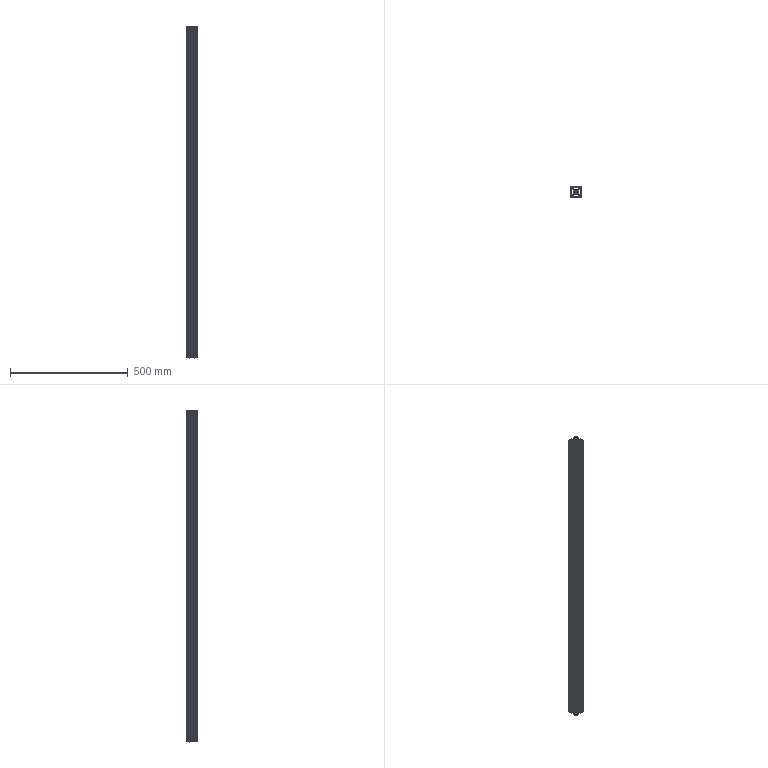Part | STEP file | 4545-1210 aluminium profile (upper long) | 1 solid | 262 faces | box 45 x 45 x 1407 mm | volume 976243 mm3 | plane 186 | cylinder 76 | commonest cylinder face diameters 2 x44 8 x20 12 x8 4 x4